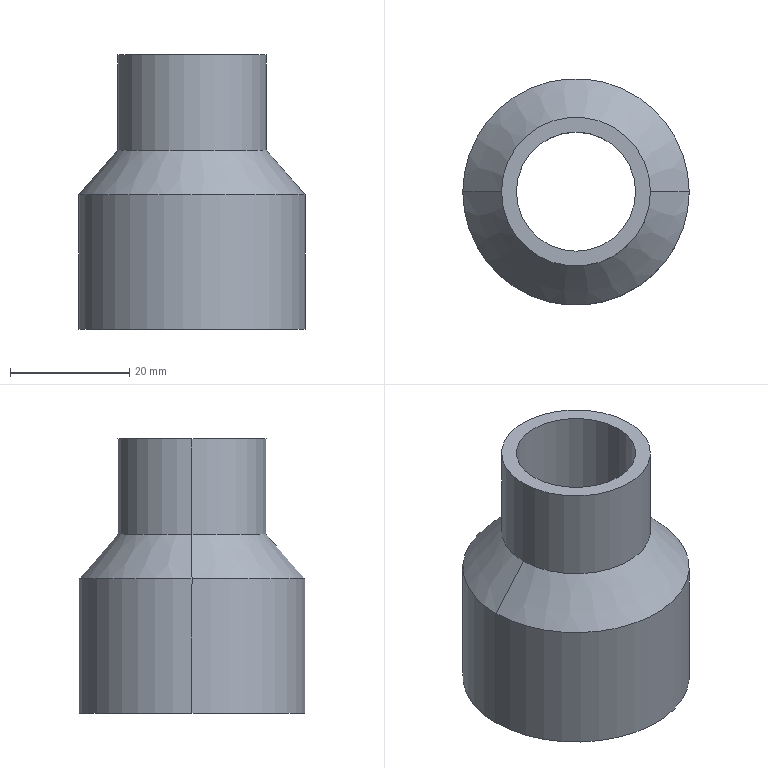Part | SolidWorks | features Revolution 1 | 1 solid | 14 faces | box 38 x 38 x 46 mm | volume 12125 mm3 | cylinder 8 | cone 4 | plane 2 | commonest cylinder face diameters 20 x2 25 x2 32 x2 38 x2
STEP:
#1=CARTESIAN_POINT('',(-10.,0.,-69.611));
#2=VERTEX_POINT('',#1);
#3=CARTESIAN_POINT('',(10.,0.,-69.611));
#4=VERTEX_POINT('',#3);
#5=CARTESIAN_POINT('',(0.,0.,-69.611));
#6=DIRECTION('',(0.,0.,1.));
#7=DIRECTION('',(1.,0.,0.));
#8=AXIS2_PLACEMENT_3D('',#5,#6,#7);
#9=CIRCLE('',#8,10.);
#10=EDGE_CURVE('',#2,#4,#9,.T.);
#11=ORIENTED_EDGE('',*,*,#10,.F.);
#12=CARTESIAN_POINT('',(-10.,0.,-53.611));
#13=VERTEX_POINT('',#12);
#14=CARTESIAN_POINT('',(-10.,0.,0.));
#15=DIRECTION('',(0.,0.,1.));
#16=VECTOR('',#15,1000.);
#17=LINE('',#14,#16);
#18=EDGE_CURVE('',#2,#13,#17,.T.);
#19=ORIENTED_EDGE('',*,*,#18,.T.);
#20=CARTESIAN_POINT('',(10.,0.,-53.611));
#21=VERTEX_POINT('',#20);
#22=CARTESIAN_POINT('',(0.,0.,-53.611));
#23=DIRECTION('',(0.,0.,1.));
#24=DIRECTION('',(1.,0.,0.));
#25=AXIS2_PLACEMENT_3D('',#22,#23,#24);
#26=CIRCLE('',#25,10.);
#27=EDGE_CURVE('',#13,#21,#26,.T.);
#28=ORIENTED_EDGE('',*,*,#27,.T.);
#29=CARTESIAN_POINT('',(10.,0.,0.));
#30=DIRECTION('',(0.,0.,1.));
#31=VECTOR('',#30,1000.);
#32=LINE('',#29,#31);
#33=EDGE_CURVE('',#4,#21,#32,.T.);
#34=ORIENTED_EDGE('',*,*,#33,.F.);
#35=EDGE_LOOP('',(#11,#19,#28,#34));
#36=FACE_OUTER_BOUND('',#35,.T.);
#37=CARTESIAN_POINT('',(0.,0.,0.));
#38=DIRECTION('',(0.,0.,1.));
#39=DIRECTION('',(1.,0.,0.));
#40=AXIS2_PLACEMENT_3D('',#37,#38,#39);
#41=CYLINDRICAL_SURFACE('',#40,10.);
#42=ADVANCED_FACE('',(#36),#41,.F.);
#43=ORIENTED_EDGE('',*,*,#10,.T.);
#44=CARTESIAN_POINT('',(16.,0.,-77.111));
#45=VERTEX_POINT('',#44);
#46=CARTESIAN_POINT('',(10.,0.,-69.611));
#47=DIRECTION('',(0.6247,0.,-0.7809));
#48=VECTOR('',#47,1000.);
#49=LINE('',#46,#48);
#50=EDGE_CURVE('',#4,#45,#49,.T.);
#51=ORIENTED_EDGE('',*,*,#50,.T.);
#52=CARTESIAN_POINT('',(-16.,0.,-77.111));
#53=VERTEX_POINT('',#52);
#54=CARTESIAN_POINT('',(0.,0.,-77.111));
#55=DIRECTION('',(0.,0.,1.));
#56=DIRECTION('',(1.,0.,0.));
#57=AXIS2_PLACEMENT_3D('',#54,#55,#56);
#58=CIRCLE('',#57,16.);
#59=EDGE_CURVE('',#53,#45,#58,.T.);
#60=ORIENTED_EDGE('',*,*,#59,.F.);
#61=CARTESIAN_POINT('',(-10.,0.,-69.611));
#62=DIRECTION('',(-0.6247,0.,-0.7809));
#63=VECTOR('',#62,1000.);
#64=LINE('',#61,#63);
#65=EDGE_CURVE('',#2,#53,#64,.T.);
#66=ORIENTED_EDGE('',*,*,#65,.F.);
#67=EDGE_LOOP('',(#43,#51,#60,#66));
#68=FACE_OUTER_BOUND('',#67,.T.);
#69=CARTESIAN_POINT('',(0.,0.,-69.611));
#70=DIRECTION('',(0.,0.,-1.));
#71=DIRECTION('',(-1.,0.,0.));
#72=AXIS2_PLACEMENT_3D('',#69,#70,#71);
#73=CONICAL_SURFACE('',#72,10.,0.6747);
#74=ADVANCED_FACE('',(#68),#73,.F.);
#75=CARTESIAN_POINT('',(-16.,0.,-99.611));
#76=VERTEX_POINT('',#75);
#77=CARTESIAN_POINT('',(16.,0.,-99.611));
#78=VERTEX_POINT('',#77);
#79=CARTESIAN_POINT('',(0.,0.,-99.611));
#80=DIRECTION('',(0.,0.,1.));
#81=DIRECTION('',(1.,0.,0.));
#82=AXIS2_PLACEMENT_3D('',#79,#80,#81);
#83=CIRCLE('',#82,16.);
#84=EDGE_CURVE('',#76,#78,#83,.T.);
#85=ORIENTED_EDGE('',*,*,#84,.F.);
#86=CARTESIAN_POINT('',(-16.,0.,0.));
#87=DIRECTION('',(0.,0.,1.));
#88=VECTOR('',#87,1000.);
#89=LINE('',#86,#88);
#90=EDGE_CURVE('',#76,#53,#89,.T.);
#91=ORIENTED_EDGE('',*,*,#90,.T.);
#92=ORIENTED_EDGE('',*,*,#59,.T.);
#93=CARTESIAN_POINT('',(16.,0.,0.));
#94=DIRECTION('',(0.,0.,1.));
#95=VECTOR('',#94,1000.);
#96=LINE('',#93,#95);
#97=EDGE_CURVE('',#78,#45,#96,.T.);
#98=ORIENTED_EDGE('',*,*,#97,.F.);
#99=EDGE_LOOP('',(#85,#91,#92,#98));
#100=FACE_OUTER_BOUND('',#99,.T.);
#101=CARTESIAN_POINT('',(0.,0.,0.));
#102=DIRECTION('',(0.,0.,1.));
#103=DIRECTION('',(1.,0.,0.));
#104=AXIS2_PLACEMENT_3D('',#101,#102,#103);
#105=CYLINDRICAL_SURFACE('',#104,16.);
#106=ADVANCED_FACE('',(#100),#105,.F.);
#107=CARTESIAN_POINT('',(19.,0.,-99.611));
#108=VERTEX_POINT('',#107);
#109=CARTESIAN_POINT('',(-19.,0.,-99.611));
#110=VERTEX_POINT('',#109);
#111=CARTESIAN_POINT('',(0.,0.,-99.611));
#112=DIRECTION('',(0.,0.,1.));
#113=DIRECTION('',(1.,0.,0.));
#114=AXIS2_PLACEMENT_3D('',#111,#112,#113);
#115=CIRCLE('',#114,19.);
#116=EDGE_CURVE('',#108,#110,#115,.T.);
#117=ORIENTED_EDGE('',*,*,#116,.T.);
#118=CARTESIAN_POINT('',(-19.,0.,-77.111));
#119=VERTEX_POINT('',#118);
#120=CARTESIAN_POINT('',(-19.,0.,0.));
#121=DIRECTION('',(0.,0.,1.));
#122=VECTOR('',#121,1000.);
#123=LINE('',#120,#122);
#124=EDGE_CURVE('',#110,#119,#123,.T.);
#125=ORIENTED_EDGE('',*,*,#124,.T.);
#126=CARTESIAN_POINT('',(19.,0.,-77.111));
#127=VERTEX_POINT('',#126);
#128=CARTESIAN_POINT('',(0.,0.,-77.111));
#129=DIRECTION('',(0.,0.,1.));
#130=DIRECTION('',(1.,0.,0.));
#131=AXIS2_PLACEMENT_3D('',#128,#129,#130);
#132=CIRCLE('',#131,19.);
#133=EDGE_CURVE('',#127,#119,#132,.T.);
#134=ORIENTED_EDGE('',*,*,#133,.F.);
#135=CARTESIAN_POINT('',(19.,0.,0.));
#136=DIRECTION('',(0.,0.,1.));
#137=VECTOR('',#136,1000.);
#138=LINE('',#135,#137);
#139=EDGE_CURVE('',#108,#127,#138,.T.);
#140=ORIENTED_EDGE('',*,*,#139,.F.);
#141=EDGE_LOOP('',(#117,#125,#134,#140));
#142=FACE_OUTER_BOUND('',#141,.T.);
#143=CARTESIAN_POINT('',(0.,0.,0.));
#144=DIRECTION('',(0.,0.,1.));
#145=DIRECTION('',(1.,0.,0.));
#146=AXIS2_PLACEMENT_3D('',#143,#144,#145);
#147=CYLINDRICAL_SURFACE('',#146,19.);
#148=ADVANCED_FACE('',(#142),#147,.T.);
#149=CARTESIAN_POINT('',(12.5,0.,-69.611));
#150=VERTEX_POINT('',#149);
#151=CARTESIAN_POINT('',(-12.5,0.,-69.611));
#152=VERTEX_POINT('',#151);
#153=CARTESIAN_POINT('',(0.,0.,-69.611));
#154=DIRECTION('',(0.,0.,1.));
#155=DIRECTION('',(1.,0.,0.));
#156=AXIS2_PLACEMENT_3D('',#153,#154,#155);
#157=CIRCLE('',#156,12.5);
#158=EDGE_CURVE('',#150,#152,#157,.T.);
#159=ORIENTED_EDGE('',*,*,#158,.F.);
#160=CARTESIAN_POINT('',(19.,0.,-77.111));
#161=DIRECTION('',(0.6549,0.,-0.7557));
#162=VECTOR('',#161,1000.);
#163=LINE('',#160,#162);
#164=EDGE_CURVE('',#150,#127,#163,.T.);
#165=ORIENTED_EDGE('',*,*,#164,.T.);
#166=ORIENTED_EDGE('',*,*,#133,.T.);
#167=CARTESIAN_POINT('',(-19.,0.,-77.111));
#168=DIRECTION('',(-0.6549,0.,-0.7557));
#169=VECTOR('',#168,1000.);
#170=LINE('',#167,#169);
#171=EDGE_CURVE('',#152,#119,#170,.T.);
#172=ORIENTED_EDGE('',*,*,#171,.F.);
#173=EDGE_LOOP('',(#159,#165,#166,#172));
#174=FACE_OUTER_BOUND('',#173,.T.);
#175=CARTESIAN_POINT('',(0.,0.,-77.111));
#176=DIRECTION('',(0.,0.,-1.));
#177=DIRECTION('',(-1.,0.,0.));
#178=AXIS2_PLACEMENT_3D('',#175,#176,#177);
#179=CONICAL_SURFACE('',#178,19.,0.7141);
#180=ADVANCED_FACE('',(#174),#179,.T.);
#181=ORIENTED_EDGE('',*,*,#158,.T.);
#182=CARTESIAN_POINT('',(-12.5,0.,-53.611));
#183=VERTEX_POINT('',#182);
#184=CARTESIAN_POINT('',(-12.5,0.,0.));
#185=DIRECTION('',(0.,0.,1.));
#186=VECTOR('',#185,1000.);
#187=LINE('',#184,#186);
#188=EDGE_CURVE('',#152,#183,#187,.T.);
#189=ORIENTED_EDGE('',*,*,#188,.T.);
#190=CARTESIAN_POINT('',(12.5,0.,-53.611));
#191=VERTEX_POINT('',#190);
#192=CARTESIAN_POINT('',(0.,0.,-53.611));
#193=DIRECTION('',(0.,0.,1.));
#194=DIRECTION('',(1.,0.,0.));
#195=AXIS2_PLACEMENT_3D('',#192,#193,#194);
#196=CIRCLE('',#195,12.5);
#197=EDGE_CURVE('',#191,#183,#196,.T.);
#198=ORIENTED_EDGE('',*,*,#197,.F.);
#199=CARTESIAN_POINT('',(12.5,0.,0.));
#200=DIRECTION('',(0.,0.,1.));
#201=VECTOR('',#200,1000.);
#202=LINE('',#199,#201);
#203=EDGE_CURVE('',#150,#191,#202,.T.);
#204=ORIENTED_EDGE('',*,*,#203,.F.);
#205=EDGE_LOOP('',(#181,#189,#198,#204));
#206=FACE_OUTER_BOUND('',#205,.T.);
#207=CARTESIAN_POINT('',(0.,0.,0.));
#208=DIRECTION('',(0.,0.,1.));
#209=DIRECTION('',(1.,0.,0.));
#210=AXIS2_PLACEMENT_3D('',#207,#208,#209);
#211=CYLINDRICAL_SURFACE('',#210,12.5);
#212=ADVANCED_FACE('',(#206),#211,.T.);
#213=CARTESIAN_POINT('',(0.,0.,-53.611));
#214=DIRECTION('',(0.,0.,1.));
#215=DIRECTION('',(1.,0.,0.));
#216=AXIS2_PLACEMENT_3D('',#213,#214,#215);
#217=CIRCLE('',#216,10.);
#218=EDGE_CURVE('',#21,#13,#217,.T.);
#219=ORIENTED_EDGE('',*,*,#218,.F.);
#220=ORIENTED_EDGE('',*,*,#27,.F.);
#221=EDGE_LOOP('',(#219,#220));
#222=FACE_BOUND('',#221,.T.);
#223=ORIENTED_EDGE('',*,*,#197,.T.);
#224=CARTESIAN_POINT('',(0.,0.,-53.611));
#225=DIRECTION('',(0.,0.,1.));
#226=DIRECTION('',(1.,0.,0.));
#227=AXIS2_PLACEMENT_3D('',#224,#225,#226);
#228=CIRCLE('',#227,12.5);
#229=EDGE_CURVE('',#183,#191,#228,.T.);
#230=ORIENTED_EDGE('',*,*,#229,.T.);
#231=EDGE_LOOP('',(#223,#230));
#232=FACE_OUTER_BOUND('',#231,.T.);
#233=CARTESIAN_POINT('',(0.,10.,-53.611));
#234=DIRECTION('',(0.,0.,-1.));
#235=DIRECTION('',(-1.,0.,0.));
#236=AXIS2_PLACEMENT_3D('',#233,#234,#235);
#237=PLANE('',#236);
#238=ADVANCED_FACE('',(#222,#232),#237,.F.);
#239=ORIENTED_EDGE('',*,*,#188,.F.);
#240=CARTESIAN_POINT('',(0.,0.,-69.611));
#241=DIRECTION('',(0.,0.,1.));
#242=DIRECTION('',(1.,0.,0.));
#243=AXIS2_PLACEMENT_3D('',#240,#241,#242);
#244=CIRCLE('',#243,12.5);
#245=EDGE_CURVE('',#152,#150,#244,.T.);
#246=ORIENTED_EDGE('',*,*,#245,.T.);
#247=ORIENTED_EDGE('',*,*,#203,.T.);
#248=ORIENTED_EDGE('',*,*,#229,.F.);
#249=EDGE_LOOP('',(#239,#246,#247,#248));
#250=FACE_OUTER_BOUND('',#249,.T.);
#251=CARTESIAN_POINT('',(0.,0.,0.));
#252=DIRECTION('',(0.,0.,1.));
#253=DIRECTION('',(1.,0.,0.));
#254=AXIS2_PLACEMENT_3D('',#251,#252,#253);
#255=CYLINDRICAL_SURFACE('',#254,12.5);
#256=ADVANCED_FACE('',(#250),#255,.T.);
#257=ORIENTED_EDGE('',*,*,#164,.F.);
#258=ORIENTED_EDGE('',*,*,#245,.F.);
#259=ORIENTED_EDGE('',*,*,#171,.T.);
#260=CARTESIAN_POINT('',(0.,0.,-77.111));
#261=DIRECTION('',(0.,0.,1.));
#262=DIRECTION('',(1.,0.,0.));
#263=AXIS2_PLACEMENT_3D('',#260,#261,#262);
#264=CIRCLE('',#263,19.);
#265=EDGE_CURVE('',#119,#127,#264,.T.);
#266=ORIENTED_EDGE('',*,*,#265,.T.);
#267=EDGE_LOOP('',(#257,#258,#259,#266));
#268=FACE_OUTER_BOUND('',#267,.T.);
#269=CARTESIAN_POINT('',(0.,0.,-77.111));
#270=DIRECTION('',(0.,0.,-1.));
#271=DIRECTION('',(-1.,0.,0.));
#272=AXIS2_PLACEMENT_3D('',#269,#270,#271);
#273=CONICAL_SURFACE('',#272,19.,0.7141);
#274=ADVANCED_FACE('',(#268),#273,.T.);
#275=ORIENTED_EDGE('',*,*,#124,.F.);
#276=CARTESIAN_POINT('',(0.,0.,-99.611));
#277=DIRECTION('',(0.,0.,1.));
#278=DIRECTION('',(1.,0.,0.));
#279=AXIS2_PLACEMENT_3D('',#276,#277,#278);
#280=CIRCLE('',#279,19.);
#281=EDGE_CURVE('',#110,#108,#280,.T.);
#282=ORIENTED_EDGE('',*,*,#281,.T.);
#283=ORIENTED_EDGE('',*,*,#139,.T.);
#284=ORIENTED_EDGE('',*,*,#265,.F.);
#285=EDGE_LOOP('',(#275,#282,#283,#284));
#286=FACE_OUTER_BOUND('',#285,.T.);
#287=CARTESIAN_POINT('',(0.,0.,0.));
#288=DIRECTION('',(0.,0.,1.));
#289=DIRECTION('',(1.,0.,0.));
#290=AXIS2_PLACEMENT_3D('',#287,#288,#289);
#291=CYLINDRICAL_SURFACE('',#290,19.);
#292=ADVANCED_FACE('',(#286),#291,.T.);
#293=ORIENTED_EDGE('',*,*,#116,.F.);
#294=ORIENTED_EDGE('',*,*,#281,.F.);
#295=EDGE_LOOP('',(#293,#294));
#296=FACE_OUTER_BOUND('',#295,.T.);
#297=CARTESIAN_POINT('',(0.,0.,-99.611));
#298=DIRECTION('',(0.,0.,1.));
#299=DIRECTION('',(1.,0.,0.));
#300=AXIS2_PLACEMENT_3D('',#297,#298,#299);
#301=CIRCLE('',#300,16.);
#302=EDGE_CURVE('',#78,#76,#301,.T.);
#303=ORIENTED_EDGE('',*,*,#302,.T.);
#304=ORIENTED_EDGE('',*,*,#84,.T.);
#305=EDGE_LOOP('',(#303,#304));
#306=FACE_BOUND('',#305,.T.);
#307=CARTESIAN_POINT('',(0.,16.,-99.611));
#308=DIRECTION('',(0.,0.,1.));
#309=DIRECTION('',(1.,0.,0.));
#310=AXIS2_PLACEMENT_3D('',#307,#308,#309);
#311=PLANE('',#310);
#312=ADVANCED_FACE('',(#296,#306),#311,.F.);
#313=ORIENTED_EDGE('',*,*,#90,.F.);
#314=ORIENTED_EDGE('',*,*,#302,.F.);
#315=ORIENTED_EDGE('',*,*,#97,.T.);
#316=CARTESIAN_POINT('',(0.,0.,-77.111));
#317=DIRECTION('',(0.,0.,1.));
#318=DIRECTION('',(1.,0.,0.));
#319=AXIS2_PLACEMENT_3D('',#316,#317,#318);
#320=CIRCLE('',#319,16.);
#321=EDGE_CURVE('',#45,#53,#320,.T.);
#322=ORIENTED_EDGE('',*,*,#321,.T.);
#323=EDGE_LOOP('',(#313,#314,#315,#322));
#324=FACE_OUTER_BOUND('',#323,.T.);
#325=CARTESIAN_POINT('',(0.,0.,0.));
#326=DIRECTION('',(0.,0.,1.));
#327=DIRECTION('',(1.,0.,0.));
#328=AXIS2_PLACEMENT_3D('',#325,#326,#327);
#329=CYLINDRICAL_SURFACE('',#328,16.);
#330=ADVANCED_FACE('',(#324),#329,.F.);
#331=ORIENTED_EDGE('',*,*,#50,.F.);
#332=CARTESIAN_POINT('',(0.,0.,-69.611));
#333=DIRECTION('',(0.,0.,1.));
#334=DIRECTION('',(1.,0.,0.));
#335=AXIS2_PLACEMENT_3D('',#332,#333,#334);
#336=CIRCLE('',#335,10.);
#337=EDGE_CURVE('',#4,#2,#336,.T.);
#338=ORIENTED_EDGE('',*,*,#337,.T.);
#339=ORIENTED_EDGE('',*,*,#65,.T.);
#340=ORIENTED_EDGE('',*,*,#321,.F.);
#341=EDGE_LOOP('',(#331,#338,#339,#340));
#342=FACE_OUTER_BOUND('',#341,.T.);
#343=CARTESIAN_POINT('',(0.,0.,-69.611));
#344=DIRECTION('',(0.,0.,-1.));
#345=DIRECTION('',(-1.,0.,0.));
#346=AXIS2_PLACEMENT_3D('',#343,#344,#345);
#347=CONICAL_SURFACE('',#346,10.,0.6747);
#348=ADVANCED_FACE('',(#342),#347,.F.);
#349=ORIENTED_EDGE('',*,*,#18,.F.);
#350=ORIENTED_EDGE('',*,*,#337,.F.);
#351=ORIENTED_EDGE('',*,*,#33,.T.);
#352=ORIENTED_EDGE('',*,*,#218,.T.);
#353=EDGE_LOOP('',(#349,#350,#351,#352));
#354=FACE_OUTER_BOUND('',#353,.T.);
#355=CARTESIAN_POINT('',(0.,0.,0.));
#356=DIRECTION('',(0.,0.,1.));
#357=DIRECTION('',(1.,0.,0.));
#358=AXIS2_PLACEMENT_3D('',#355,#356,#357);
#359=CYLINDRICAL_SURFACE('',#358,10.);
#360=ADVANCED_FACE('',(#354),#359,.F.);
#361=CLOSED_SHELL('',(#42,#74,#106,#148,#180,#212,#238,#256,#274,#292,#312,#330,#348,#360));
#362=MANIFOLD_SOLID_BREP('',#361);
#363=CARTESIAN_POINT('',(0.,0.,0.));
#364=DIRECTION('',(0.,0.,1.));
#365=DIRECTION('',(1.,0.,0.));
#366=AXIS2_PLACEMENT_3D('',#363,#364,#365);
#367=(LENGTH_UNIT()NAMED_UNIT(*)SI_UNIT(.MILLI.,.METRE.));
#368=UNCERTAINTY_MEASURE_WITH_UNIT(LENGTH_MEASURE(0.00001),#367,'','');
#369=(NAMED_UNIT(*)PLANE_ANGLE_UNIT()SI_UNIT($,.RADIAN.));
#370=(NAMED_UNIT(*)SI_UNIT($,.STERADIAN.)SOLID_ANGLE_UNIT());
#371=(GEOMETRIC_REPRESENTATION_CONTEXT(3)GLOBAL_UNCERTAINTY_ASSIGNED_CONTEXT((#368))GLOBAL_UNIT_ASSIGNED_CONTEXT((#367,#369,#370))REPRESENTATION_CONTEXT('',''));
#372=ADVANCED_BREP_SHAPE_REPRESENTATION('',(#362,#366),#371);